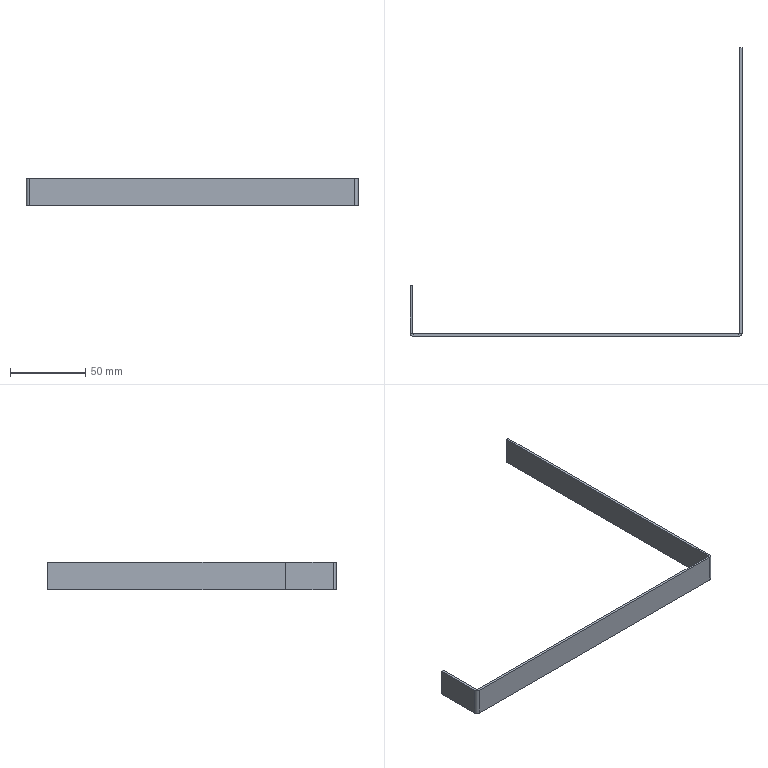Part | SolidWorks | features FlatPattern 1, SMBaseFlange 1, SheetMetal 1 | 1 solid | 22 faces | box 220 x 191 x 18.5 mm | volume 12216 mm3 | plane 18 | cylinder 4 | commonest cylinder face diameters 1 x2 4 x2
STEP:
#1=CARTESIAN_POINT('',(49.34,-82.459,18.5));
#2=VERTEX_POINT('',#1);
#3=CARTESIAN_POINT('',(50.84,-82.459,18.5));
#4=VERTEX_POINT('',#3);
#5=CARTESIAN_POINT('',(49.34,-82.459,18.5));
#6=DIRECTION('',(1.,0.,0.));
#7=VECTOR('',#6,1000.);
#8=LINE('',#5,#7);
#9=EDGE_CURVE('',#2,#4,#8,.T.);
#10=ORIENTED_EDGE('',*,*,#9,.F.);
#11=CARTESIAN_POINT('',(51.34,-84.459,18.5));
#12=VERTEX_POINT('',#11);
#13=CARTESIAN_POINT('',(51.34,-82.459,18.5));
#14=DIRECTION('',(0.,0.,1.));
#15=DIRECTION('',(-1.,0.,0.));
#16=AXIS2_PLACEMENT_3D('',#13,#14,#15);
#17=CIRCLE('',#16,2.);
#18=EDGE_CURVE('',#2,#12,#17,.T.);
#19=ORIENTED_EDGE('',*,*,#18,.T.);
#20=CARTESIAN_POINT('',(51.34,-82.959,18.5));
#21=VERTEX_POINT('',#20);
#22=CARTESIAN_POINT('',(51.34,-82.959,18.5));
#23=DIRECTION('',(0.,-1.,0.));
#24=VECTOR('',#23,1000.);
#25=LINE('',#22,#24);
#26=EDGE_CURVE('',#21,#12,#25,.T.);
#27=ORIENTED_EDGE('',*,*,#26,.F.);
#28=CARTESIAN_POINT('',(51.34,-82.459,18.5));
#29=DIRECTION('',(0.,0.,1.));
#30=DIRECTION('',(1.,0.,0.));
#31=AXIS2_PLACEMENT_3D('',#28,#29,#30);
#32=CIRCLE('',#31,0.5);
#33=EDGE_CURVE('',#4,#21,#32,.T.);
#34=ORIENTED_EDGE('',*,*,#33,.F.);
#35=EDGE_LOOP('',(#10,#19,#27,#34));
#36=FACE_OUTER_BOUND('',#35,.T.);
#37=CARTESIAN_POINT('',(49.34,-82.459,18.5));
#38=DIRECTION('',(0.,0.,1.));
#39=DIRECTION('',(1.,0.,0.));
#40=AXIS2_PLACEMENT_3D('',#37,#38,#39);
#41=PLANE('',#40);
#42=ADVANCED_FACE('',(#36),#41,.T.);
#43=CARTESIAN_POINT('',(49.34,-51.159,18.5));
#44=VERTEX_POINT('',#43);
#45=CARTESIAN_POINT('',(49.34,-51.159,18.5));
#46=DIRECTION('',(0.,-1.,0.));
#47=VECTOR('',#46,1000.);
#48=LINE('',#45,#47);
#49=EDGE_CURVE('',#44,#2,#48,.T.);
#50=ORIENTED_EDGE('',*,*,#49,.T.);
#51=ORIENTED_EDGE('',*,*,#9,.T.);
#52=CARTESIAN_POINT('',(50.84,-51.159,18.5));
#53=VERTEX_POINT('',#52);
#54=CARTESIAN_POINT('',(50.84,-51.159,18.5));
#55=DIRECTION('',(0.,-1.,0.));
#56=VECTOR('',#55,1000.);
#57=LINE('',#54,#56);
#58=EDGE_CURVE('',#53,#4,#57,.T.);
#59=ORIENTED_EDGE('',*,*,#58,.F.);
#60=CARTESIAN_POINT('',(49.34,-51.159,18.5));
#61=DIRECTION('',(1.,0.,0.));
#62=VECTOR('',#61,1000.);
#63=LINE('',#60,#62);
#64=EDGE_CURVE('',#44,#53,#63,.T.);
#65=ORIENTED_EDGE('',*,*,#64,.F.);
#66=EDGE_LOOP('',(#50,#51,#59,#65));
#67=FACE_OUTER_BOUND('',#66,.T.);
#68=CARTESIAN_POINT('',(51.34,-82.959,18.5));
#69=DIRECTION('',(0.,0.,1.));
#70=DIRECTION('',(1.,0.,0.));
#71=AXIS2_PLACEMENT_3D('',#68,#69,#70);
#72=PLANE('',#71);
#73=ADVANCED_FACE('',(#67),#72,.T.);
#74=CARTESIAN_POINT('',(51.34,-84.459,0.));
#75=VERTEX_POINT('',#74);
#76=CARTESIAN_POINT('',(51.34,-82.959,0.));
#77=VERTEX_POINT('',#76);
#78=CARTESIAN_POINT('',(51.34,-84.459,0.));
#79=DIRECTION('',(0.,1.,0.));
#80=VECTOR('',#79,1000.);
#81=LINE('',#78,#80);
#82=EDGE_CURVE('',#75,#77,#81,.T.);
#83=ORIENTED_EDGE('',*,*,#82,.F.);
#84=CARTESIAN_POINT('',(49.34,-82.459,0.));
#85=VERTEX_POINT('',#84);
#86=CARTESIAN_POINT('',(51.34,-82.459,0.));
#87=DIRECTION('',(0.,0.,1.));
#88=DIRECTION('',(-1.,0.,0.));
#89=AXIS2_PLACEMENT_3D('',#86,#87,#88);
#90=CIRCLE('',#89,2.);
#91=EDGE_CURVE('',#85,#75,#90,.T.);
#92=ORIENTED_EDGE('',*,*,#91,.F.);
#93=CARTESIAN_POINT('',(50.84,-82.459,0.));
#94=VERTEX_POINT('',#93);
#95=CARTESIAN_POINT('',(50.84,-82.459,0.));
#96=DIRECTION('',(-1.,0.,0.));
#97=VECTOR('',#96,1000.);
#98=LINE('',#95,#97);
#99=EDGE_CURVE('',#94,#85,#98,.T.);
#100=ORIENTED_EDGE('',*,*,#99,.F.);
#101=CARTESIAN_POINT('',(51.34,-82.459,0.));
#102=DIRECTION('',(0.,0.,1.));
#103=DIRECTION('',(1.,0.,0.));
#104=AXIS2_PLACEMENT_3D('',#101,#102,#103);
#105=CIRCLE('',#104,0.5);
#106=EDGE_CURVE('',#94,#77,#105,.T.);
#107=ORIENTED_EDGE('',*,*,#106,.T.);
#108=EDGE_LOOP('',(#83,#92,#100,#107));
#109=FACE_OUTER_BOUND('',#108,.T.);
#110=CARTESIAN_POINT('',(51.34,-84.459,0.));
#111=DIRECTION('',(0.,0.,-1.));
#112=DIRECTION('',(-1.,0.,0.));
#113=AXIS2_PLACEMENT_3D('',#110,#111,#112);
#114=PLANE('',#113);
#115=ADVANCED_FACE('',(#109),#114,.T.);
#116=CARTESIAN_POINT('',(267.34,-84.459,0.));
#117=VERTEX_POINT('',#116);
#118=CARTESIAN_POINT('',(49.34,-84.459,0.));
#119=DIRECTION('',(1.,0.,0.));
#120=VECTOR('',#119,1000.);
#121=LINE('',#118,#120);
#122=EDGE_CURVE('',#75,#117,#121,.T.);
#123=ORIENTED_EDGE('',*,*,#122,.F.);
#124=ORIENTED_EDGE('',*,*,#82,.T.);
#125=CARTESIAN_POINT('',(267.34,-82.959,0.));
#126=VERTEX_POINT('',#125);
#127=CARTESIAN_POINT('',(49.34,-82.959,0.));
#128=DIRECTION('',(1.,0.,0.));
#129=VECTOR('',#128,1000.);
#130=LINE('',#127,#129);
#131=EDGE_CURVE('',#77,#126,#130,.T.);
#132=ORIENTED_EDGE('',*,*,#131,.T.);
#133=CARTESIAN_POINT('',(267.34,-82.959,0.));
#134=DIRECTION('',(0.,-1.,0.));
#135=VECTOR('',#134,1000.);
#136=LINE('',#133,#135);
#137=EDGE_CURVE('',#126,#117,#136,.T.);
#138=ORIENTED_EDGE('',*,*,#137,.T.);
#139=EDGE_LOOP('',(#123,#124,#132,#138));
#140=FACE_OUTER_BOUND('',#139,.T.);
#141=CARTESIAN_POINT('',(50.84,-82.459,0.));
#142=DIRECTION('',(0.,0.,-1.));
#143=DIRECTION('',(-1.,0.,0.));
#144=AXIS2_PLACEMENT_3D('',#141,#142,#143);
#145=PLANE('',#144);
#146=ADVANCED_FACE('',(#140),#145,.T.);
#147=CARTESIAN_POINT('',(267.34,-84.459,18.5));
#148=VERTEX_POINT('',#147);
#149=CARTESIAN_POINT('',(267.34,-82.959,18.5));
#150=VERTEX_POINT('',#149);
#151=CARTESIAN_POINT('',(267.34,-84.459,18.5));
#152=DIRECTION('',(0.,1.,0.));
#153=VECTOR('',#152,1000.);
#154=LINE('',#151,#153);
#155=EDGE_CURVE('',#148,#150,#154,.T.);
#156=ORIENTED_EDGE('',*,*,#155,.F.);
#157=CARTESIAN_POINT('',(269.34,-82.459,18.5));
#158=VERTEX_POINT('',#157);
#159=CARTESIAN_POINT('',(267.34,-82.459,18.5));
#160=DIRECTION('',(0.,0.,1.));
#161=DIRECTION('',(-1.,0.,0.));
#162=AXIS2_PLACEMENT_3D('',#159,#160,#161);
#163=CIRCLE('',#162,2.);
#164=EDGE_CURVE('',#148,#158,#163,.T.);
#165=ORIENTED_EDGE('',*,*,#164,.T.);
#166=CARTESIAN_POINT('',(267.84,-82.459,18.5));
#167=VERTEX_POINT('',#166);
#168=CARTESIAN_POINT('',(267.84,-82.459,18.5));
#169=DIRECTION('',(1.,0.,0.));
#170=VECTOR('',#169,1000.);
#171=LINE('',#168,#170);
#172=EDGE_CURVE('',#167,#158,#171,.T.);
#173=ORIENTED_EDGE('',*,*,#172,.F.);
#174=CARTESIAN_POINT('',(267.34,-82.459,18.5));
#175=DIRECTION('',(0.,0.,1.));
#176=DIRECTION('',(1.,0.,0.));
#177=AXIS2_PLACEMENT_3D('',#174,#175,#176);
#178=CIRCLE('',#177,0.5);
#179=EDGE_CURVE('',#150,#167,#178,.T.);
#180=ORIENTED_EDGE('',*,*,#179,.F.);
#181=EDGE_LOOP('',(#156,#165,#173,#180));
#182=FACE_OUTER_BOUND('',#181,.T.);
#183=CARTESIAN_POINT('',(267.34,-84.459,18.5));
#184=DIRECTION('',(0.,0.,1.));
#185=DIRECTION('',(1.,0.,0.));
#186=AXIS2_PLACEMENT_3D('',#183,#184,#185);
#187=PLANE('',#186);
#188=ADVANCED_FACE('',(#182),#187,.T.);
#189=CARTESIAN_POINT('',(49.34,-84.459,18.5));
#190=DIRECTION('',(1.,0.,0.));
#191=VECTOR('',#190,1000.);
#192=LINE('',#189,#191);
#193=EDGE_CURVE('',#12,#148,#192,.T.);
#194=ORIENTED_EDGE('',*,*,#193,.T.);
#195=ORIENTED_EDGE('',*,*,#155,.T.);
#196=CARTESIAN_POINT('',(49.34,-82.959,18.5));
#197=DIRECTION('',(1.,0.,0.));
#198=VECTOR('',#197,1000.);
#199=LINE('',#196,#198);
#200=EDGE_CURVE('',#21,#150,#199,.T.);
#201=ORIENTED_EDGE('',*,*,#200,.F.);
#202=ORIENTED_EDGE('',*,*,#26,.T.);
#203=EDGE_LOOP('',(#194,#195,#201,#202));
#204=FACE_OUTER_BOUND('',#203,.T.);
#205=CARTESIAN_POINT('',(267.84,-82.459,18.5));
#206=DIRECTION('',(0.,0.,1.));
#207=DIRECTION('',(1.,0.,0.));
#208=AXIS2_PLACEMENT_3D('',#205,#206,#207);
#209=PLANE('',#208);
#210=ADVANCED_FACE('',(#204),#209,.T.);
#211=CARTESIAN_POINT('',(269.34,-82.459,0.));
#212=VERTEX_POINT('',#211);
#213=CARTESIAN_POINT('',(267.84,-82.459,0.));
#214=VERTEX_POINT('',#213);
#215=CARTESIAN_POINT('',(269.34,-82.459,0.));
#216=DIRECTION('',(-1.,0.,0.));
#217=VECTOR('',#216,1000.);
#218=LINE('',#215,#217);
#219=EDGE_CURVE('',#212,#214,#218,.T.);
#220=ORIENTED_EDGE('',*,*,#219,.F.);
#221=CARTESIAN_POINT('',(267.34,-82.459,0.));
#222=DIRECTION('',(0.,0.,1.));
#223=DIRECTION('',(-1.,0.,0.));
#224=AXIS2_PLACEMENT_3D('',#221,#222,#223);
#225=CIRCLE('',#224,2.);
#226=EDGE_CURVE('',#117,#212,#225,.T.);
#227=ORIENTED_EDGE('',*,*,#226,.F.);
#228=ORIENTED_EDGE('',*,*,#137,.F.);
#229=CARTESIAN_POINT('',(267.34,-82.459,0.));
#230=DIRECTION('',(0.,0.,1.));
#231=DIRECTION('',(1.,0.,0.));
#232=AXIS2_PLACEMENT_3D('',#229,#230,#231);
#233=CIRCLE('',#232,0.5);
#234=EDGE_CURVE('',#126,#214,#233,.T.);
#235=ORIENTED_EDGE('',*,*,#234,.T.);
#236=EDGE_LOOP('',(#220,#227,#228,#235));
#237=FACE_OUTER_BOUND('',#236,.T.);
#238=CARTESIAN_POINT('',(269.34,-82.459,0.));
#239=DIRECTION('',(0.,0.,-1.));
#240=DIRECTION('',(-1.,0.,0.));
#241=AXIS2_PLACEMENT_3D('',#238,#239,#240);
#242=PLANE('',#241);
#243=ADVANCED_FACE('',(#237),#242,.T.);
#244=CARTESIAN_POINT('',(269.34,106.541,0.));
#245=VERTEX_POINT('',#244);
#246=CARTESIAN_POINT('',(269.34,-84.459,0.));
#247=DIRECTION('',(0.,1.,0.));
#248=VECTOR('',#247,1000.);
#249=LINE('',#246,#248);
#250=EDGE_CURVE('',#212,#245,#249,.T.);
#251=ORIENTED_EDGE('',*,*,#250,.F.);
#252=ORIENTED_EDGE('',*,*,#219,.T.);
#253=CARTESIAN_POINT('',(267.84,106.541,0.));
#254=VERTEX_POINT('',#253);
#255=CARTESIAN_POINT('',(267.84,-84.459,0.));
#256=DIRECTION('',(0.,1.,0.));
#257=VECTOR('',#256,1000.);
#258=LINE('',#255,#257);
#259=EDGE_CURVE('',#214,#254,#258,.T.);
#260=ORIENTED_EDGE('',*,*,#259,.T.);
#261=CARTESIAN_POINT('',(267.84,106.541,0.));
#262=DIRECTION('',(1.,0.,0.));
#263=VECTOR('',#262,1000.);
#264=LINE('',#261,#263);
#265=EDGE_CURVE('',#254,#245,#264,.T.);
#266=ORIENTED_EDGE('',*,*,#265,.T.);
#267=EDGE_LOOP('',(#251,#252,#260,#266));
#268=FACE_OUTER_BOUND('',#267,.T.);
#269=CARTESIAN_POINT('',(267.34,-82.959,0.));
#270=DIRECTION('',(0.,0.,-1.));
#271=DIRECTION('',(-1.,0.,0.));
#272=AXIS2_PLACEMENT_3D('',#269,#270,#271);
#273=PLANE('',#272);
#274=ADVANCED_FACE('',(#268),#273,.T.);
#275=ORIENTED_EDGE('',*,*,#250,.T.);
#276=CARTESIAN_POINT('',(269.34,106.541,18.5));
#277=VERTEX_POINT('',#276);
#278=CARTESIAN_POINT('',(269.34,106.541,18.5));
#279=DIRECTION('',(0.,0.,-1.));
#280=VECTOR('',#279,1000.);
#281=LINE('',#278,#280);
#282=EDGE_CURVE('',#277,#245,#281,.T.);
#283=ORIENTED_EDGE('',*,*,#282,.F.);
#284=CARTESIAN_POINT('',(269.34,-84.459,18.5));
#285=DIRECTION('',(0.,1.,0.));
#286=VECTOR('',#285,1000.);
#287=LINE('',#284,#286);
#288=EDGE_CURVE('',#158,#277,#287,.T.);
#289=ORIENTED_EDGE('',*,*,#288,.F.);
#290=CARTESIAN_POINT('',(269.34,-82.459,18.5));
#291=DIRECTION('',(0.,0.,-1.));
#292=VECTOR('',#291,1000.);
#293=LINE('',#290,#292);
#294=EDGE_CURVE('',#158,#212,#293,.T.);
#295=ORIENTED_EDGE('',*,*,#294,.T.);
#296=EDGE_LOOP('',(#275,#283,#289,#295));
#297=FACE_OUTER_BOUND('',#296,.T.);
#298=CARTESIAN_POINT('',(269.34,-84.459,18.5));
#299=DIRECTION('',(-1.,0.,0.));
#300=DIRECTION('',(0.,0.,1.));
#301=AXIS2_PLACEMENT_3D('',#298,#299,#300);
#302=PLANE('',#301);
#303=ADVANCED_FACE('',(#297),#302,.F.);
#304=ORIENTED_EDGE('',*,*,#265,.F.);
#305=CARTESIAN_POINT('',(267.84,106.541,18.5));
#306=VERTEX_POINT('',#305);
#307=CARTESIAN_POINT('',(267.84,106.541,18.5));
#308=DIRECTION('',(0.,0.,-1.));
#309=VECTOR('',#308,1000.);
#310=LINE('',#307,#309);
#311=EDGE_CURVE('',#306,#254,#310,.T.);
#312=ORIENTED_EDGE('',*,*,#311,.F.);
#313=CARTESIAN_POINT('',(267.84,106.541,18.5));
#314=DIRECTION('',(1.,0.,0.));
#315=VECTOR('',#314,1000.);
#316=LINE('',#313,#315);
#317=EDGE_CURVE('',#306,#277,#316,.T.);
#318=ORIENTED_EDGE('',*,*,#317,.T.);
#319=ORIENTED_EDGE('',*,*,#282,.T.);
#320=EDGE_LOOP('',(#304,#312,#318,#319));
#321=FACE_OUTER_BOUND('',#320,.T.);
#322=CARTESIAN_POINT('',(267.84,106.541,18.5));
#323=DIRECTION('',(0.,1.,0.));
#324=DIRECTION('',(0.,0.,1.));
#325=AXIS2_PLACEMENT_3D('',#322,#323,#324);
#326=PLANE('',#325);
#327=ADVANCED_FACE('',(#321),#326,.T.);
#328=ORIENTED_EDGE('',*,*,#259,.F.);
#329=CARTESIAN_POINT('',(267.84,-82.459,18.5));
#330=DIRECTION('',(0.,0.,-1.));
#331=VECTOR('',#330,1000.);
#332=LINE('',#329,#331);
#333=EDGE_CURVE('',#167,#214,#332,.T.);
#334=ORIENTED_EDGE('',*,*,#333,.F.);
#335=CARTESIAN_POINT('',(267.84,-84.459,18.5));
#336=DIRECTION('',(0.,1.,0.));
#337=VECTOR('',#336,1000.);
#338=LINE('',#335,#337);
#339=EDGE_CURVE('',#167,#306,#338,.T.);
#340=ORIENTED_EDGE('',*,*,#339,.T.);
#341=ORIENTED_EDGE('',*,*,#311,.T.);
#342=EDGE_LOOP('',(#328,#334,#340,#341));
#343=FACE_OUTER_BOUND('',#342,.T.);
#344=CARTESIAN_POINT('',(267.84,-84.459,18.5));
#345=DIRECTION('',(-1.,0.,0.));
#346=DIRECTION('',(0.,0.,1.));
#347=AXIS2_PLACEMENT_3D('',#344,#345,#346);
#348=PLANE('',#347);
#349=ADVANCED_FACE('',(#343),#348,.T.);
#350=ORIENTED_EDGE('',*,*,#234,.F.);
#351=CARTESIAN_POINT('',(267.34,-82.959,18.5));
#352=DIRECTION('',(0.,0.,-1.));
#353=VECTOR('',#352,1000.);
#354=LINE('',#351,#353);
#355=EDGE_CURVE('',#150,#126,#354,.T.);
#356=ORIENTED_EDGE('',*,*,#355,.F.);
#357=ORIENTED_EDGE('',*,*,#179,.T.);
#358=ORIENTED_EDGE('',*,*,#333,.T.);
#359=EDGE_LOOP('',(#350,#356,#357,#358));
#360=FACE_OUTER_BOUND('',#359,.T.);
#361=CARTESIAN_POINT('',(267.34,-82.459,18.5));
#362=DIRECTION('',(0.,0.,-1.));
#363=DIRECTION('',(-1.,0.,0.));
#364=AXIS2_PLACEMENT_3D('',#361,#362,#363);
#365=CYLINDRICAL_SURFACE('',#364,0.5);
#366=ADVANCED_FACE('',(#360),#365,.F.);
#367=ORIENTED_EDGE('',*,*,#131,.F.);
#368=CARTESIAN_POINT('',(51.34,-82.959,18.5));
#369=DIRECTION('',(0.,0.,-1.));
#370=VECTOR('',#369,1000.);
#371=LINE('',#368,#370);
#372=EDGE_CURVE('',#21,#77,#371,.T.);
#373=ORIENTED_EDGE('',*,*,#372,.F.);
#374=ORIENTED_EDGE('',*,*,#200,.T.);
#375=ORIENTED_EDGE('',*,*,#355,.T.);
#376=EDGE_LOOP('',(#367,#373,#374,#375));
#377=FACE_OUTER_BOUND('',#376,.T.);
#378=CARTESIAN_POINT('',(49.34,-82.959,18.5));
#379=DIRECTION('',(0.,1.,0.));
#380=DIRECTION('',(0.,0.,1.));
#381=AXIS2_PLACEMENT_3D('',#378,#379,#380);
#382=PLANE('',#381);
#383=ADVANCED_FACE('',(#377),#382,.T.);
#384=ORIENTED_EDGE('',*,*,#106,.F.);
#385=CARTESIAN_POINT('',(50.84,-82.459,18.5));
#386=DIRECTION('',(0.,0.,-1.));
#387=VECTOR('',#386,1000.);
#388=LINE('',#385,#387);
#389=EDGE_CURVE('',#4,#94,#388,.T.);
#390=ORIENTED_EDGE('',*,*,#389,.F.);
#391=ORIENTED_EDGE('',*,*,#33,.T.);
#392=ORIENTED_EDGE('',*,*,#372,.T.);
#393=EDGE_LOOP('',(#384,#390,#391,#392));
#394=FACE_OUTER_BOUND('',#393,.T.);
#395=CARTESIAN_POINT('',(51.34,-82.459,18.5));
#396=DIRECTION('',(0.,0.,-1.));
#397=DIRECTION('',(-1.,0.,0.));
#398=AXIS2_PLACEMENT_3D('',#395,#396,#397);
#399=CYLINDRICAL_SURFACE('',#398,0.5);
#400=ADVANCED_FACE('',(#394),#399,.F.);
#401=CARTESIAN_POINT('',(50.84,-51.159,0.));
#402=VERTEX_POINT('',#401);
#403=CARTESIAN_POINT('',(50.84,-51.159,0.));
#404=DIRECTION('',(0.,-1.,0.));
#405=VECTOR('',#404,1000.);
#406=LINE('',#403,#405);
#407=EDGE_CURVE('',#402,#94,#406,.T.);
#408=ORIENTED_EDGE('',*,*,#407,.F.);
#409=CARTESIAN_POINT('',(50.84,-51.159,18.5));
#410=DIRECTION('',(0.,0.,-1.));
#411=VECTOR('',#410,1000.);
#412=LINE('',#409,#411);
#413=EDGE_CURVE('',#53,#402,#412,.T.);
#414=ORIENTED_EDGE('',*,*,#413,.F.);
#415=ORIENTED_EDGE('',*,*,#58,.T.);
#416=ORIENTED_EDGE('',*,*,#389,.T.);
#417=EDGE_LOOP('',(#408,#414,#415,#416));
#418=FACE_OUTER_BOUND('',#417,.T.);
#419=CARTESIAN_POINT('',(50.84,-51.159,18.5));
#420=DIRECTION('',(1.,0.,0.));
#421=DIRECTION('',(0.,1.,0.));
#422=AXIS2_PLACEMENT_3D('',#419,#420,#421);
#423=PLANE('',#422);
#424=ADVANCED_FACE('',(#418),#423,.T.);
#425=CARTESIAN_POINT('',(49.34,-51.159,0.));
#426=VERTEX_POINT('',#425);
#427=CARTESIAN_POINT('',(49.34,-51.159,0.));
#428=DIRECTION('',(1.,0.,0.));
#429=VECTOR('',#428,1000.);
#430=LINE('',#427,#429);
#431=EDGE_CURVE('',#426,#402,#430,.T.);
#432=ORIENTED_EDGE('',*,*,#431,.F.);
#433=CARTESIAN_POINT('',(49.34,-51.159,18.5));
#434=DIRECTION('',(0.,0.,-1.));
#435=VECTOR('',#434,1000.);
#436=LINE('',#433,#435);
#437=EDGE_CURVE('',#44,#426,#436,.T.);
#438=ORIENTED_EDGE('',*,*,#437,.F.);
#439=ORIENTED_EDGE('',*,*,#64,.T.);
#440=ORIENTED_EDGE('',*,*,#413,.T.);
#441=EDGE_LOOP('',(#432,#438,#439,#440));
#442=FACE_OUTER_BOUND('',#441,.T.);
#443=CARTESIAN_POINT('',(49.34,-51.159,18.5));
#444=DIRECTION('',(0.,1.,0.));
#445=DIRECTION('',(0.,0.,1.));
#446=AXIS2_PLACEMENT_3D('',#443,#444,#445);
#447=PLANE('',#446);
#448=ADVANCED_FACE('',(#442),#447,.T.);
#449=CARTESIAN_POINT('',(49.34,-51.159,0.));
#450=DIRECTION('',(0.,-1.,0.));
#451=VECTOR('',#450,1000.);
#452=LINE('',#449,#451);
#453=EDGE_CURVE('',#426,#85,#452,.T.);
#454=ORIENTED_EDGE('',*,*,#453,.T.);
#455=CARTESIAN_POINT('',(49.34,-82.459,18.5));
#456=DIRECTION('',(0.,0.,-1.));
#457=VECTOR('',#456,1000.);
#458=LINE('',#455,#457);
#459=EDGE_CURVE('',#2,#85,#458,.T.);
#460=ORIENTED_EDGE('',*,*,#459,.F.);
#461=ORIENTED_EDGE('',*,*,#49,.F.);
#462=ORIENTED_EDGE('',*,*,#437,.T.);
#463=EDGE_LOOP('',(#454,#460,#461,#462));
#464=FACE_OUTER_BOUND('',#463,.T.);
#465=CARTESIAN_POINT('',(49.34,-51.159,18.5));
#466=DIRECTION('',(1.,0.,0.));
#467=DIRECTION('',(0.,1.,0.));
#468=AXIS2_PLACEMENT_3D('',#465,#466,#467);
#469=PLANE('',#468);
#470=ADVANCED_FACE('',(#464),#469,.F.);
#471=ORIENTED_EDGE('',*,*,#91,.T.);
#472=CARTESIAN_POINT('',(51.34,-84.459,18.5));
#473=DIRECTION('',(0.,0.,-1.));
#474=VECTOR('',#473,1000.);
#475=LINE('',#472,#474);
#476=EDGE_CURVE('',#12,#75,#475,.T.);
#477=ORIENTED_EDGE('',*,*,#476,.F.);
#478=ORIENTED_EDGE('',*,*,#18,.F.);
#479=ORIENTED_EDGE('',*,*,#459,.T.);
#480=EDGE_LOOP('',(#471,#477,#478,#479));
#481=FACE_OUTER_BOUND('',#480,.T.);
#482=CARTESIAN_POINT('',(51.34,-82.459,18.5));
#483=DIRECTION('',(0.,0.,-1.));
#484=DIRECTION('',(-1.,0.,0.));
#485=AXIS2_PLACEMENT_3D('',#482,#483,#484);
#486=CYLINDRICAL_SURFACE('',#485,2.);
#487=ADVANCED_FACE('',(#481),#486,.T.);
#488=ORIENTED_EDGE('',*,*,#122,.T.);
#489=CARTESIAN_POINT('',(267.34,-84.459,18.5));
#490=DIRECTION('',(0.,0.,-1.));
#491=VECTOR('',#490,1000.);
#492=LINE('',#489,#491);
#493=EDGE_CURVE('',#148,#117,#492,.T.);
#494=ORIENTED_EDGE('',*,*,#493,.F.);
#495=ORIENTED_EDGE('',*,*,#193,.F.);
#496=ORIENTED_EDGE('',*,*,#476,.T.);
#497=EDGE_LOOP('',(#488,#494,#495,#496));
#498=FACE_OUTER_BOUND('',#497,.T.);
#499=CARTESIAN_POINT('',(49.34,-84.459,18.5));
#500=DIRECTION('',(0.,1.,0.));
#501=DIRECTION('',(0.,0.,1.));
#502=AXIS2_PLACEMENT_3D('',#499,#500,#501);
#503=PLANE('',#502);
#504=ADVANCED_FACE('',(#498),#503,.F.);
#505=ORIENTED_EDGE('',*,*,#226,.T.);
#506=ORIENTED_EDGE('',*,*,#294,.F.);
#507=ORIENTED_EDGE('',*,*,#164,.F.);
#508=ORIENTED_EDGE('',*,*,#493,.T.);
#509=EDGE_LOOP('',(#505,#506,#507,#508));
#510=FACE_OUTER_BOUND('',#509,.T.);
#511=CARTESIAN_POINT('',(267.34,-82.459,18.5));
#512=DIRECTION('',(0.,0.,-1.));
#513=DIRECTION('',(-1.,0.,0.));
#514=AXIS2_PLACEMENT_3D('',#511,#512,#513);
#515=CYLINDRICAL_SURFACE('',#514,2.);
#516=ADVANCED_FACE('',(#510),#515,.T.);
#517=ORIENTED_EDGE('',*,*,#288,.T.);
#518=ORIENTED_EDGE('',*,*,#317,.F.);
#519=ORIENTED_EDGE('',*,*,#339,.F.);
#520=ORIENTED_EDGE('',*,*,#172,.T.);
#521=EDGE_LOOP('',(#517,#518,#519,#520));
#522=FACE_OUTER_BOUND('',#521,.T.);
#523=CARTESIAN_POINT('',(267.34,-82.459,18.5));
#524=DIRECTION('',(0.,0.,1.));
#525=DIRECTION('',(1.,0.,0.));
#526=AXIS2_PLACEMENT_3D('',#523,#524,#525);
#527=PLANE('',#526);
#528=ADVANCED_FACE('',(#522),#527,.T.);
#529=ORIENTED_EDGE('',*,*,#407,.T.);
#530=ORIENTED_EDGE('',*,*,#99,.T.);
#531=ORIENTED_EDGE('',*,*,#453,.F.);
#532=ORIENTED_EDGE('',*,*,#431,.T.);
#533=EDGE_LOOP('',(#529,#530,#531,#532));
#534=FACE_OUTER_BOUND('',#533,.T.);
#535=CARTESIAN_POINT('',(267.34,-82.459,0.));
#536=DIRECTION('',(0.,0.,1.));
#537=DIRECTION('',(1.,0.,0.));
#538=AXIS2_PLACEMENT_3D('',#535,#536,#537);
#539=PLANE('',#538);
#540=ADVANCED_FACE('',(#534),#539,.F.);
#541=CLOSED_SHELL('',(#42,#73,#115,#146,#188,#210,#243,#274,#303,#327,#349,#366,#383,#400,#424,#448,#470,#487,#504,#516,#528,#540));
#542=MANIFOLD_SOLID_BREP('',#541);
#543=CARTESIAN_POINT('',(0.,0.,0.));
#544=DIRECTION('',(0.,0.,1.));
#545=DIRECTION('',(1.,0.,0.));
#546=AXIS2_PLACEMENT_3D('',#543,#544,#545);
#547=(LENGTH_UNIT()NAMED_UNIT(*)SI_UNIT(.MILLI.,.METRE.));
#548=UNCERTAINTY_MEASURE_WITH_UNIT(LENGTH_MEASURE(0.00001),#547,'','');
#549=(NAMED_UNIT(*)PLANE_ANGLE_UNIT()SI_UNIT($,.RADIAN.));
#550=(NAMED_UNIT(*)SI_UNIT($,.STERADIAN.)SOLID_ANGLE_UNIT());
#551=(GEOMETRIC_REPRESENTATION_CONTEXT(3)GLOBAL_UNCERTAINTY_ASSIGNED_CONTEXT((#548))GLOBAL_UNIT_ASSIGNED_CONTEXT((#547,#549,#550))REPRESENTATION_CONTEXT('',''));
#552=ADVANCED_BREP_SHAPE_REPRESENTATION('',(#542,#546),#551);